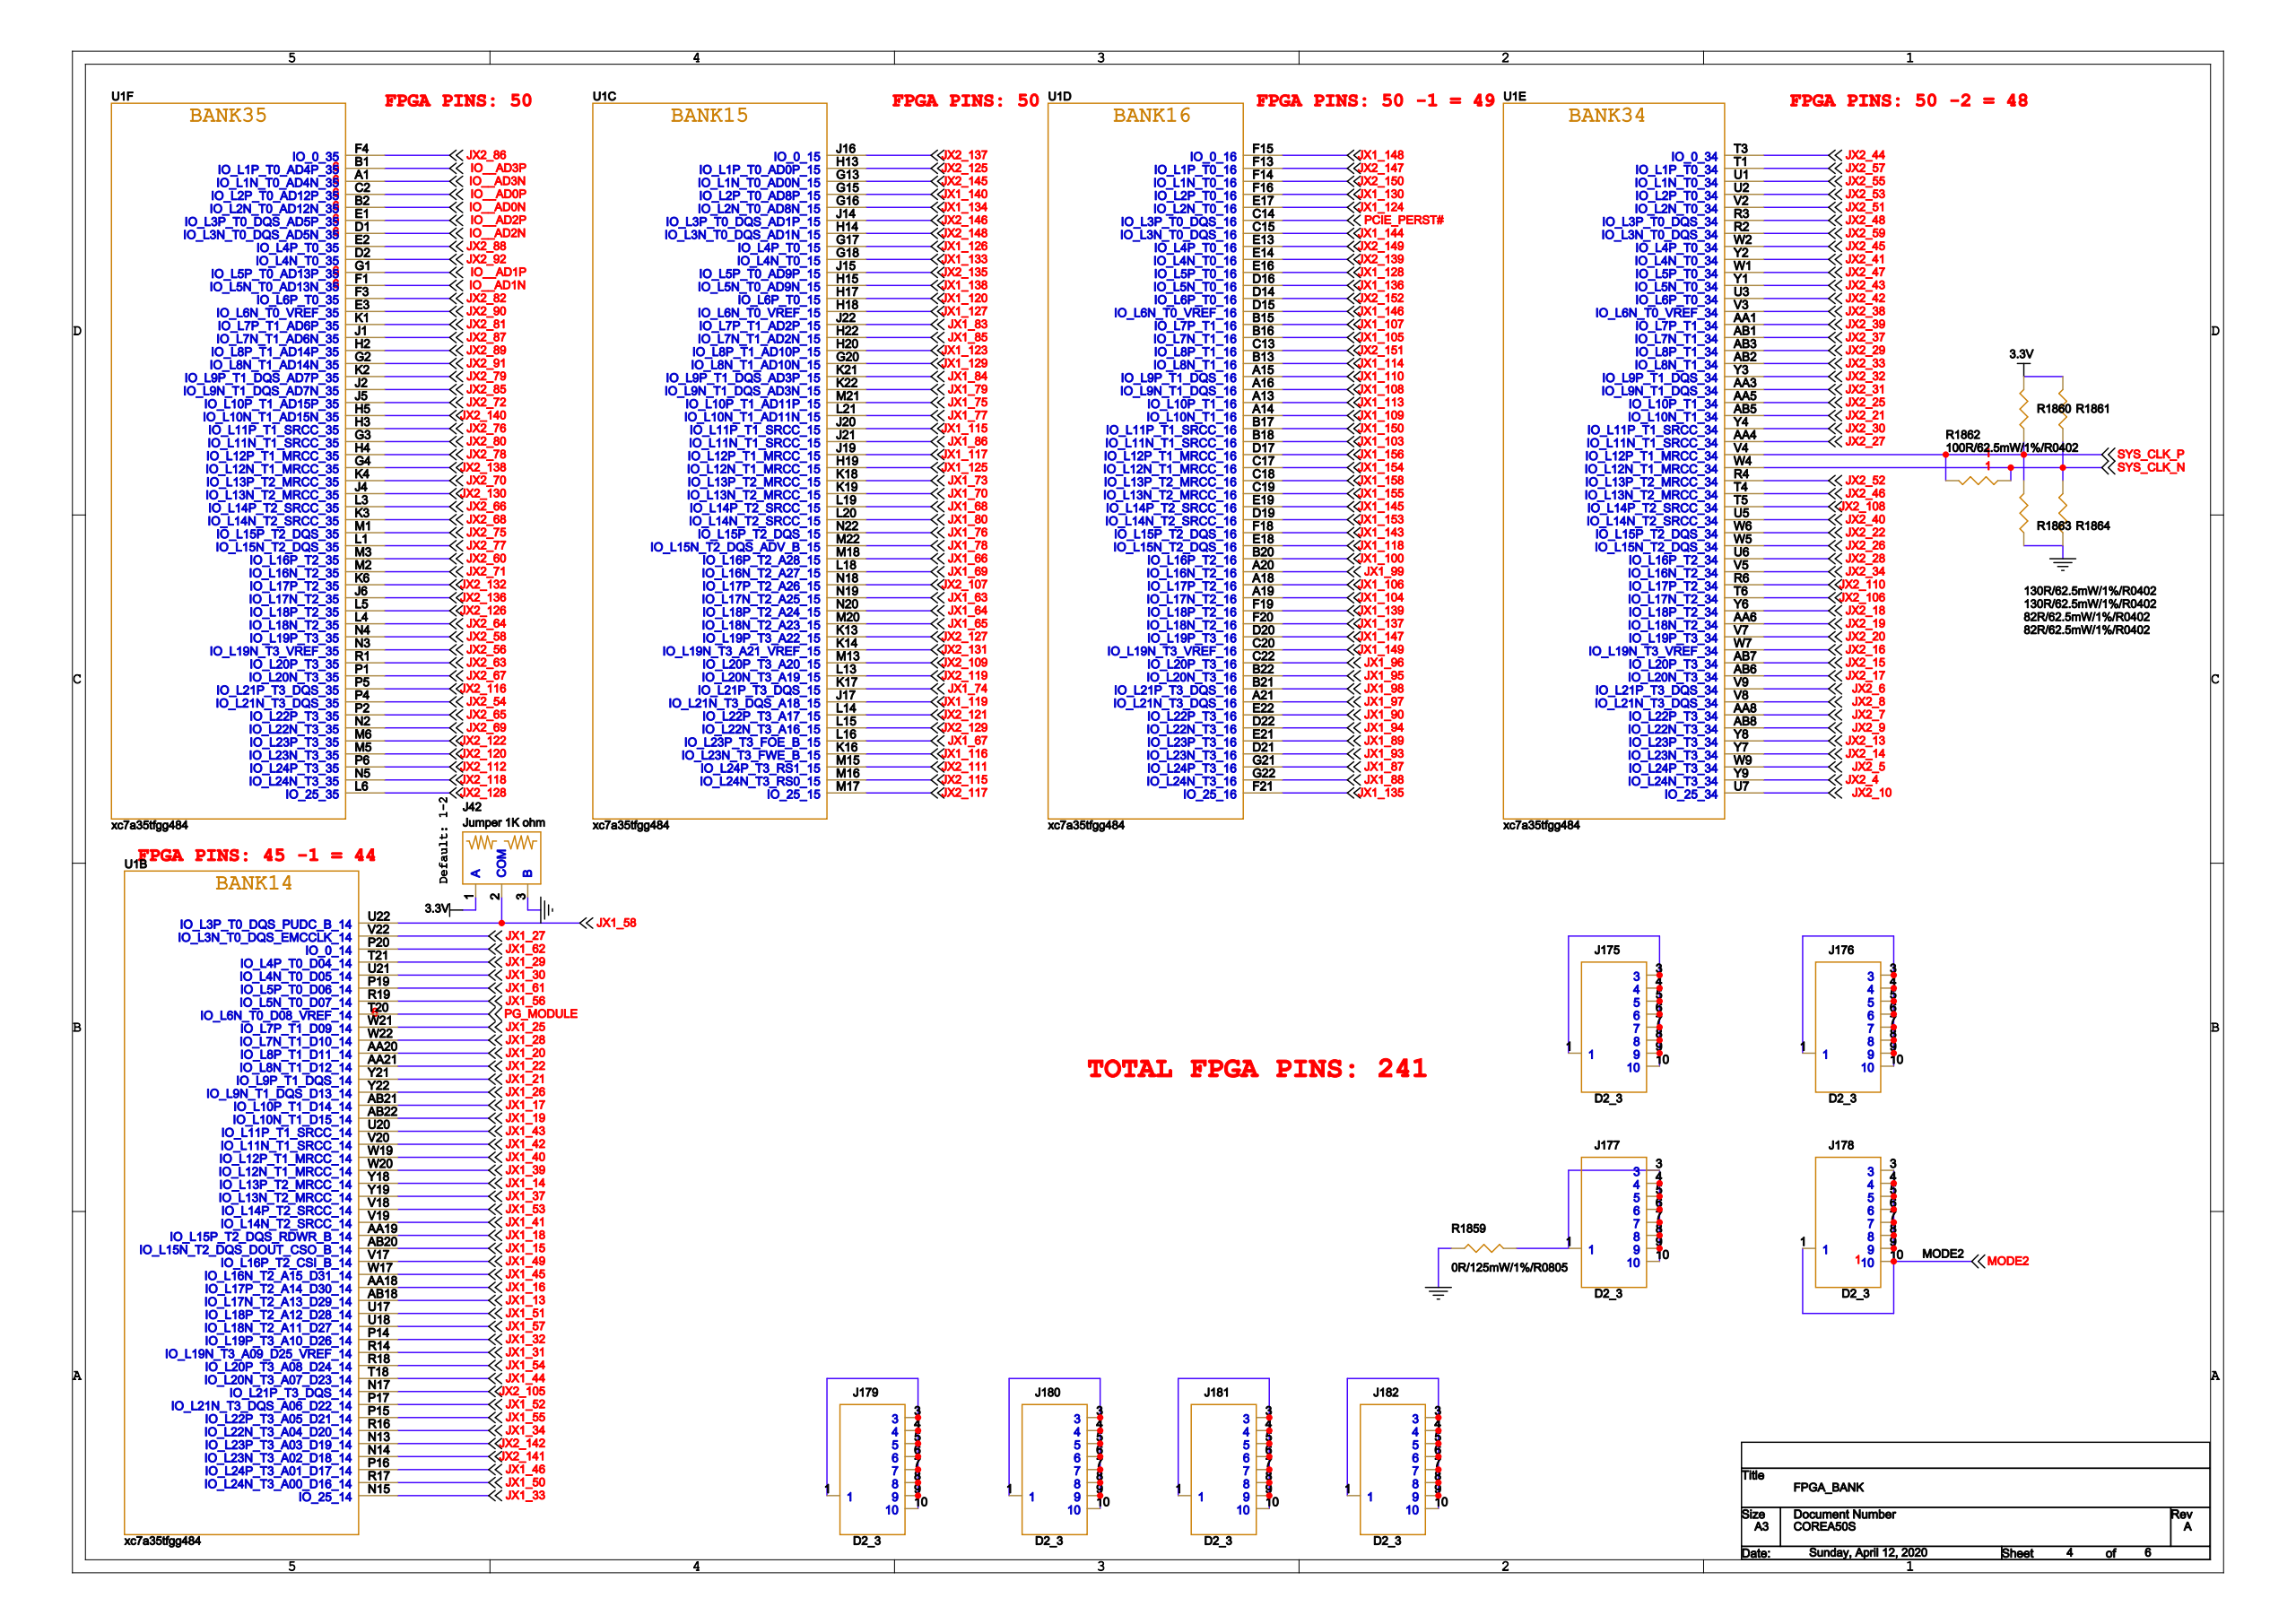Circuit board | Cadence Allegro | 202 parts | 354 nets | one sheet of the schematic
Parts on this sheet (reference | value | footprint):
J42 | Jumper 1K ohm | 0402-3P
J175 | D2_3 | D2_3
J176 | D2_3 | D2_3
J177 | D2_3 | D2_3
J178 | D2_3 | D2_3
J179 | D2_3 | D2_3
J180 | D2_3 | D2_3
J181 | D2_3 | D2_3
J182 | D2_3 | D2_3
R1859 | 0R/125mW/1%/R0805 | 0805
R1860 | 130R/62.5mW/1%/R0402 | 0402
R1861 | 130R/62.5mW/1%/R0402 | 0402
R1862 | 100R/62.5mW/1%/R0402 | 0402
R1863 | 82R/62.5mW/1%/R0402 | 0402
R1864 | 82R/62.5mW/1%/R0402 | 0402
U1 | xc7a35tfgg484 | FGG484_23X23
Nets of these parts (net: part-pin ...):
GND: J42-3 R1859-2 R1863-2 R1864-2 U1-A3
3.3V: J42-1 R1860-1 R1861-1
PCIE_PERST#: U1-C14
JX1_27: U1-V22
JX1_58: J42-2 U1-U22
MODE2: J178-1 J178-3 J178-4 J178-5 J178-6 J178-7 J178-8 J178-9 J178-10
JX1_62: U1-P20
JX1_33: U1-N15
JX1_19: U1-AB22
JX1_17: U1-AB21
JX1_42: U1-V20
JX1_43: U1-U20
JX1_39: U1-W20
JX1_40: U1-W19
JX1_37: U1-Y19
JX1_14: U1-Y18
JX1_41: U1-V19
JX1_53: U1-V18
JX1_15: U1-AB20
JX1_18: U1-AA19
JX1_45: U1-W17
JX1_49: U1-V17
JX1_13: U1-AB18
JX1_16: U1-AA18
JX1_57: U1-U18
JX1_51: U1-U17
JX1_31: U1-R14
JX1_32: U1-P14
JX1_44: U1-T18
JX1_54: U1-R18
JX1_52: U1-P17
JX2_105: U1-N17
JX1_34: U1-R16
JX1_55: U1-P15
JX2_141: U1-N14
JX2_142: U1-N13
JX1_50: U1-R17
JX1_46: U1-P16
JX1_30: U1-U21
JX1_29: U1-T21
JX1_56: U1-R19
JX1_61: U1-P19
PG_MODULE: U1-T20
JX1_28: U1-W22
JX1_25: U1-W21
JX1_22: U1-AA21
JX1_20: U1-AA20
JX1_26: U1-Y22
JX1_21: U1-Y21
JX2_137: U1-J16
JX2_117: U1-M17
JX1_77: U1-L21
JX1_75: U1-M21
JX1_86: U1-J21
JX1_115: U1-J20
JX1_125: U1-H19
JX1_117: U1-J19
JX1_70: U1-K19
JX1_73: U1-K18
JX1_80: U1-L20
JX1_68: U1-L19
JX1_78: U1-M22
JX1_76: U1-N22
JX1_69: U1-L18
JX1_66: U1-M18
JX1_63: U1-N19
JX2_107: U1-N18
JX1_65: U1-M20
JX1_64: U1-N20
JX2_131: U1-K14
JX2_127: U1-K13
JX2_145: U1-G13
JX2_125: U1-H13
JX2_119: U1-L13
JX2_109: U1-M13
JX1_119: U1-J17
JX1_74: U1-K17
JX2_129: U1-L15
JX2_121: U1-L14
JX1_116: U1-K16
JX1_67: U1-L16
JX2_115: U1-M16
JX2_111: U1-M15
JX1_134: U1-G16
JX1_140: U1-G15
JX2_148: U1-H14
JX2_146: U1-J14
JX1_133: U1-G18
JX1_126: U1-G17
JX1_138: U1-H15
JX2_135: U1-J15
JX1_127: U1-H18
JX1_120: U1-H17
JX1_85: U1-H22
JX1_83: U1-J22
JX1_129: U1-G20
JX1_123: U1-H20
JX1_79: U1-K22
JX1_84: U1-K21
JX1_148: U1-F15
JX1_135: U1-F21
JX1_109: U1-A14
JX1_113: U1-A13
JX1_103: U1-B18
JX1_150: U1-B17
JX1_154: U1-C17
JX1_156: U1-D17
JX1_155: U1-C19
JX1_158: U1-C18
JX1_153: U1-D19
JX1_145: U1-E19
JX1_118: U1-E18
JX1_143: U1-F18
JX1_99: U1-A20
JX1_100: U1-B20
JX1_104: U1-A19
JX1_106: U1-A18
JX1_137: U1-F20
JX1_139: U1-F19
JX1_149: U1-C20
JX1_147: U1-D20
JX2_150: U1-F14
JX2_147: U1-F13
JX1_95: U1-B22
JX1_96: U1-C22
JX1_97: U1-A21
JX1_98: U1-B21
JX1_94: U1-D22
JX1_90: U1-E22
JX1_93: U1-D21
JX1_89: U1-E21
JX1_88: U1-G22
JX1_87: U1-G21
JX1_124: U1-E17
JX1_130: U1-F16
JX1_144: U1-C15
JX2_139: U1-E14
JX2_149: U1-E13
JX1_136: U1-D16
JX1_128: U1-E16
JX1_146: U1-D15
JX2_152: U1-D14
JX1_105: U1-B16
JX1_107: U1-B15
JX1_114: U1-B13
JX2_151: U1-C13
JX1_108: U1-A16
JX1_110: U1-A15
JX2_44: U1-T3
JX2_10: U1-U7
JX2_21: U1-AB5
JX2_25: U1-AA5
JX2_27: U1-AA4
JX2_30: U1-Y4
SYS_CLK_N: R1861-2 R1862-2 R1864-1 U1-W4
SYS_CLK_P: R1860-2 R1862-1 R1863-1 U1-V4
JX2_46: U1-T4
JX2_52: U1-R4
JX2_40: U1-U5
JX2_108: U1-T5
JX2_26: U1-W5
JX2_22: U1-W6
JX2_34: U1-V5
JX2_28: U1-U6
JX2_106: U1-T6
JX2_110: U1-R6
JX2_19: U1-AA6
JX2_18: U1-Y6
JX2_16: U1-W7
JX2_20: U1-V7
JX2_55: U1-U1
JX2_57: U1-T1
JX2_17: U1-AB6
JX2_15: U1-AB7
JX2_8: U1-V8
JX2_6: U1-V9
JX2_9: U1-AB8
JX2_7: U1-AA8
JX2_14: U1-Y7
JX2_13: U1-Y8
JX2_4: U1-Y9
JX2_5: U1-W9
JX2_51: U1-V2
JX2_53: U1-U2
JX2_59: U1-R2
JX2_48: U1-R3
JX2_41: U1-Y2
JX2_45: U1-W2
JX2_43: U1-Y1
JX2_47: U1-W1
JX2_38: U1-V3
JX2_42: U1-U3
JX2_37: U1-AB1
JX2_39: U1-AA1
JX2_33: U1-AB2
JX2_29: U1-AB3
JX2_31: U1-AA3
JX2_32: U1-Y3
JX2_86: U1-F4
JX2_128: U1-L6
JX2_140: U1-H5
JX2_72: U1-J5
JX2_80: U1-G3
JX2_76: U1-H3
JX2_138: U1-G4
JX2_78: U1-H4
JX2_130: U1-J4
JX2_70: U1-K4
JX2_68: U1-K3
JX2_66: U1-L3
JX2_77: U1-L1
JX2_75: U1-M1
JX2_71: U1-M2
JX2_60: U1-M3
JX2_136: U1-J6
JX2_132: U1-K6
JX2_64: U1-L4
JX2_126: U1-L5
JX2_56: U1-N3
JX2_58: U1-N4
IO__AD3N: U1-A1
IO__AD3P: U1-B1
JX2_67: U1-P1
JX2_63: U1-R1
JX2_54: U1-P4
JX2_116: U1-P5
JX2_69: U1-N2
JX2_65: U1-P2
JX2_120: U1-M5
JX2_122: U1-M6
JX2_118: U1-N5
JX2_112: U1-P6
IO__AD0N: U1-B2
IO__AD0P: U1-C2
IO__AD2N: U1-D1
IO__AD2P: U1-E1
JX2_92: U1-D2
JX2_88: U1-E2
IO__AD1N: U1-F1
IO__AD1P: U1-G1
JX2_90: U1-E3
JX2_82: U1-F3
JX2_87: U1-J1
JX2_81: U1-K1
JX2_91: U1-G2
JX2_89: U1-H2
JX2_85: U1-J2
JX2_79: U1-K2
N26239706: J177-1 J177-3 J177-4 J177-5 J177-6 J177-7 J177-8 J177-9 J177-10 R1859-1
N26391692: J179-1 J179-3 J179-4 J179-5 J179-6 J179-7 J179-8 J179-9 J179-10
N26391738: J180-1 J180-3 J180-4 J180-5 J180-6 J180-7 J180-8 J180-9 J180-10
N26391784: J181-1 J181-3 J181-4 J181-5 J181-6 J181-7 J181-8 J181-9 J181-10
N26391830: J182-1 J182-3 J182-4 J182-5 J182-6 J182-7 J182-8 J182-9 J182-10
N26239664: J175-1 J175-3 J175-4 J175-5 J175-6 J175-7 J175-8 J175-9 J175-10
N26239670: J176-1 J176-3 J176-4 J176-5 J176-6 J176-7 J176-8 J176-9 J176-10